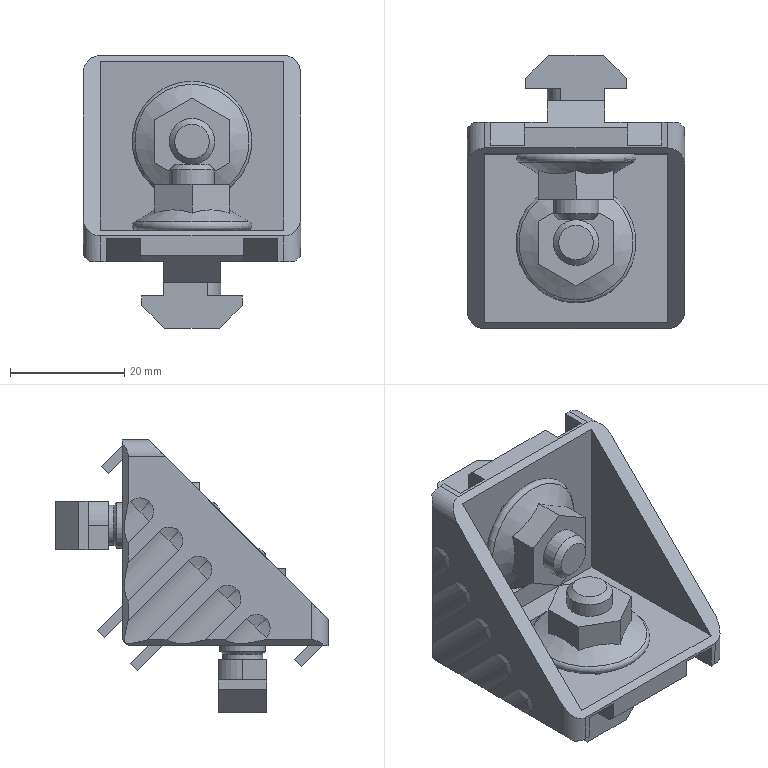Part | STEP file | bosch_3842529383_ce331vk4hpgd1h6tci1llkgc1 | 1 solid | 214 faces | box 38 x 47.7 x 47.7 mm | volume 18640 mm3 | plane 158 | cylinder 24 | spline 20 | cone 10 | torus 2 | commonest cylinder face diameters 9.151 x5 9.512 x5 6 x4 8 x4 10 x4 7 x2